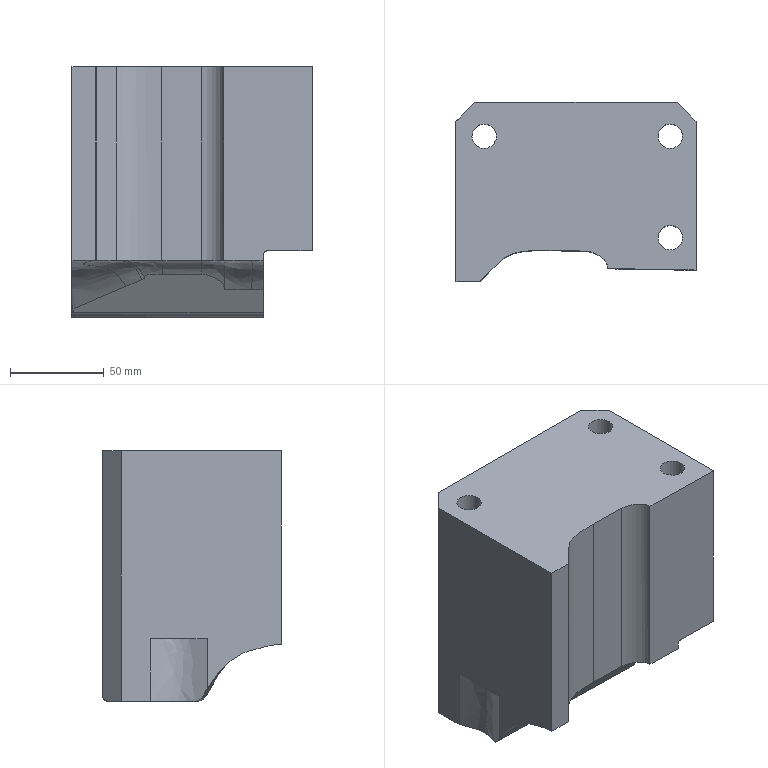Part | NX | features solid 2 | 1 solid | 47 faces | box 127.709 x 95.155 x 133.25 mm | volume 1223192 mm3 | plane 19 | cylinder 14 | spline 12 | cone 2 | commonest cylinder face diameters 13 x3 20 x3 4 x1 6 x1 8.5 x1 10 x1